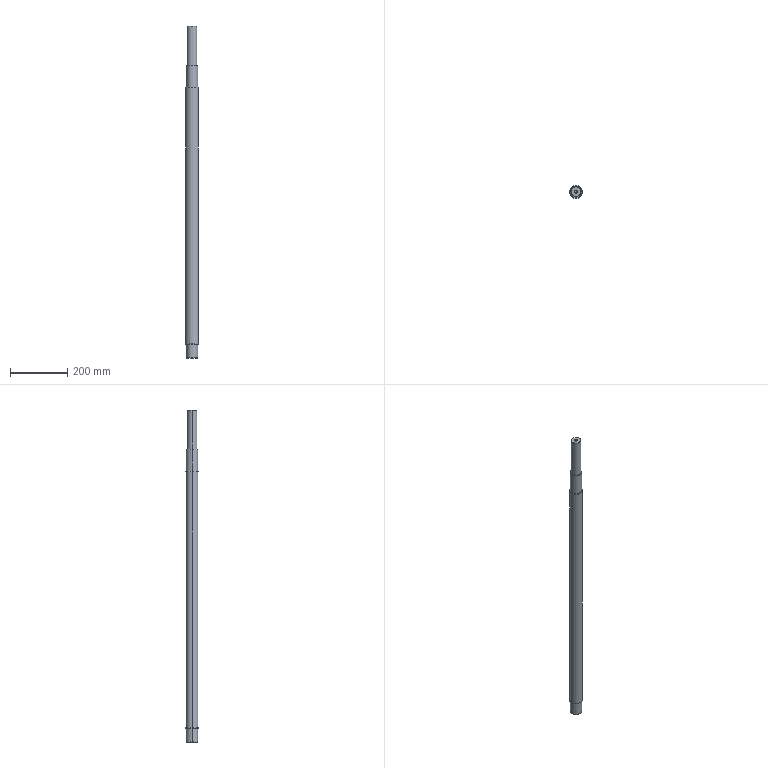Part | SolidWorks | features ICE 4, Chamfer 2, HoleWzd 2, Extrusion 1, Fillet 1 | 1 solid | 39 faces | box 45 x 45 x 1164 mm | volume 1714375 mm3 | cylinder 15 | cone 14 | plane 8 | torus 2 | commonest cylinder face diameters 40 x4 10 x3 8.5 x2 10.2 x2 35 x2 45 x2
STEP:
#1=CARTESIAN_POINT('',(-21.,0.,0.));
#2=VERTEX_POINT('',#1);
#3=CARTESIAN_POINT('',(21.,0.,0.));
#4=VERTEX_POINT('',#3);
#5=CARTESIAN_POINT('',(0.,0.,0.));
#6=DIRECTION('',(0.,0.,1.));
#7=DIRECTION('',(1.,0.,0.));
#8=AXIS2_PLACEMENT_3D('',#5,#6,#7);
#9=CIRCLE('',#8,21.);
#10=EDGE_CURVE('',#2,#4,#9,.T.);
#11=ORIENTED_EDGE('',*,*,#10,.F.);
#12=CARTESIAN_POINT('',(-20.,0.,-1.));
#13=VERTEX_POINT('',#12);
#14=CARTESIAN_POINT('',(-21.,0.,-1.));
#15=DIRECTION('',(0.,1.,0.));
#16=DIRECTION('',(-1.,0.,0.));
#17=AXIS2_PLACEMENT_3D('',#14,#15,#16);
#18=CIRCLE('',#17,1.);
#19=EDGE_CURVE('',#2,#13,#18,.T.);
#20=ORIENTED_EDGE('',*,*,#19,.T.);
#21=CARTESIAN_POINT('',(20.,0.,-1.));
#22=VERTEX_POINT('',#21);
#23=CARTESIAN_POINT('',(0.,0.,-1.));
#24=DIRECTION('',(0.,0.,-1.));
#25=DIRECTION('',(1.,0.,0.));
#26=AXIS2_PLACEMENT_3D('',#23,#24,#25);
#27=CIRCLE('',#26,20.);
#28=EDGE_CURVE('',#22,#13,#27,.T.);
#29=ORIENTED_EDGE('',*,*,#28,.F.);
#30=CARTESIAN_POINT('',(21.,0.,-1.));
#31=DIRECTION('',(0.,-1.,0.));
#32=DIRECTION('',(0.,0.,-1.));
#33=AXIS2_PLACEMENT_3D('',#30,#31,#32);
#34=CIRCLE('',#33,1.);
#35=EDGE_CURVE('',#4,#22,#34,.T.);
#36=ORIENTED_EDGE('',*,*,#35,.F.);
#37=EDGE_LOOP('',(#11,#20,#29,#36));
#38=FACE_OUTER_BOUND('',#37,.T.);
#39=CARTESIAN_POINT('',(0.,0.,-1.));
#40=DIRECTION('',(0.,0.,1.));
#41=DIRECTION('',(1.,0.,0.));
#42=AXIS2_PLACEMENT_3D('',#39,#40,#41);
#43=TOROIDAL_SURFACE('',#42,21.,1.);
#44=ADVANCED_FACE('',(#38),#43,.F.);
#45=CARTESIAN_POINT('',(-22.098,0.,0.));
#46=VERTEX_POINT('',#45);
#47=CARTESIAN_POINT('',(22.098,0.,0.));
#48=VERTEX_POINT('',#47);
#49=CARTESIAN_POINT('',(0.,0.,0.));
#50=DIRECTION('',(0.,0.,-1.));
#51=DIRECTION('',(1.,0.,0.));
#52=AXIS2_PLACEMENT_3D('',#49,#50,#51);
#53=CIRCLE('',#52,22.098);
#54=EDGE_CURVE('',#46,#48,#53,.T.);
#55=ORIENTED_EDGE('',*,*,#54,.F.);
#56=CARTESIAN_POINT('',(-22.5,0.,1.5));
#57=VERTEX_POINT('',#56);
#58=CARTESIAN_POINT('',(-22.5,0.,1.5));
#59=DIRECTION('',(-0.2588,0.,0.9659));
#60=VECTOR('',#59,1000.);
#61=LINE('',#58,#60);
#62=EDGE_CURVE('',#46,#57,#61,.T.);
#63=ORIENTED_EDGE('',*,*,#62,.T.);
#64=CARTESIAN_POINT('',(22.5,0.,1.5));
#65=VERTEX_POINT('',#64);
#66=CARTESIAN_POINT('',(0.,0.,1.5));
#67=DIRECTION('',(0.,0.,1.));
#68=DIRECTION('',(1.,0.,0.));
#69=AXIS2_PLACEMENT_3D('',#66,#67,#68);
#70=CIRCLE('',#69,22.5);
#71=EDGE_CURVE('',#65,#57,#70,.T.);
#72=ORIENTED_EDGE('',*,*,#71,.F.);
#73=CARTESIAN_POINT('',(22.5,0.,1.5));
#74=DIRECTION('',(0.2588,0.,0.9659));
#75=VECTOR('',#74,1000.);
#76=LINE('',#73,#75);
#77=EDGE_CURVE('',#48,#65,#76,.T.);
#78=ORIENTED_EDGE('',*,*,#77,.F.);
#79=EDGE_LOOP('',(#55,#63,#72,#78));
#80=FACE_OUTER_BOUND('',#79,.T.);
#81=CARTESIAN_POINT('',(0.,0.,1.5));
#82=DIRECTION('',(0.,0.,1.));
#83=DIRECTION('',(1.,0.,0.));
#84=AXIS2_PLACEMENT_3D('',#81,#82,#83);
#85=CONICAL_SURFACE('',#84,22.5,0.2618);
#86=ADVANCED_FACE('',(#80),#85,.T.);
#87=CARTESIAN_POINT('',(4.25,0.,-24.));
#88=VERTEX_POINT('',#87);
#89=CARTESIAN_POINT('',(-4.25,0.,-24.));
#90=VERTEX_POINT('',#89);
#91=CARTESIAN_POINT('',(0.,0.,-24.));
#92=DIRECTION('',(0.,0.,-1.));
#93=DIRECTION('',(-1.,0.,0.));
#94=AXIS2_PLACEMENT_3D('',#91,#92,#93);
#95=CIRCLE('',#94,4.25);
#96=EDGE_CURVE('',#88,#90,#95,.T.);
#97=ORIENTED_EDGE('',*,*,#96,.F.);
#98=CARTESIAN_POINT('',(4.25,0.,-48.5));
#99=VERTEX_POINT('',#98);
#100=CARTESIAN_POINT('',(4.25,0.,-48.5));
#101=DIRECTION('',(0.,0.,-1.));
#102=VECTOR('',#101,1000.);
#103=LINE('',#100,#102);
#104=EDGE_CURVE('',#88,#99,#103,.T.);
#105=ORIENTED_EDGE('',*,*,#104,.T.);
#106=CARTESIAN_POINT('',(-4.25,0.,-48.5));
#107=VERTEX_POINT('',#106);
#108=CARTESIAN_POINT('',(0.,0.,-48.5));
#109=DIRECTION('',(0.,0.,-1.));
#110=DIRECTION('',(-1.,0.,0.));
#111=AXIS2_PLACEMENT_3D('',#108,#109,#110);
#112=CIRCLE('',#111,4.25);
#113=EDGE_CURVE('',#99,#107,#112,.T.);
#114=ORIENTED_EDGE('',*,*,#113,.T.);
#115=CARTESIAN_POINT('',(-4.25,0.,-48.5));
#116=DIRECTION('',(0.,0.,-1.));
#117=VECTOR('',#116,1000.);
#118=LINE('',#115,#117);
#119=EDGE_CURVE('',#90,#107,#118,.T.);
#120=ORIENTED_EDGE('',*,*,#119,.F.);
#121=EDGE_LOOP('',(#97,#105,#114,#120));
#122=FACE_OUTER_BOUND('',#121,.T.);
#123=CARTESIAN_POINT('',(0.,0.,-48.5));
#124=DIRECTION('',(0.,0.,-1.));
#125=DIRECTION('',(-1.,0.,0.));
#126=AXIS2_PLACEMENT_3D('',#123,#124,#125);
#127=CYLINDRICAL_SURFACE('',#126,4.25);
#128=ADVANCED_FACE('',(#122),#127,.F.);
#129=CARTESIAN_POINT('',(0.,0.,-21.446));
#130=VERTEX_POINT('',#129);
#131=CARTESIAN_POINT('',(-4.25,0.,-24.));
#132=DIRECTION('',(-0.8572,0.,-0.515));
#133=VECTOR('',#132,1000.);
#134=LINE('',#131,#133);
#135=EDGE_CURVE('',#130,#90,#134,.T.);
#136=ORIENTED_EDGE('',*,*,#135,.F.);
#137=CARTESIAN_POINT('',(4.25,0.,-24.));
#138=DIRECTION('',(0.8572,0.,-0.515));
#139=VECTOR('',#138,1000.);
#140=LINE('',#137,#139);
#141=EDGE_CURVE('',#130,#88,#140,.T.);
#142=ORIENTED_EDGE('',*,*,#141,.T.);
#143=ORIENTED_EDGE('',*,*,#96,.T.);
#144=EDGE_LOOP('',(#136,#142,#143));
#145=FACE_OUTER_BOUND('',#144,.T.);
#146=CARTESIAN_POINT('',(0.,0.,-24.));
#147=DIRECTION('',(0.,0.,-1.));
#148=DIRECTION('',(-1.,0.,0.));
#149=AXIS2_PLACEMENT_3D('',#146,#147,#148);
#150=CONICAL_SURFACE('',#149,4.25,1.03);
#151=ADVANCED_FACE('',(#145),#150,.F.);
#152=CARTESIAN_POINT('',(-5.1,0.,1085.75));
#153=VERTEX_POINT('',#152);
#154=CARTESIAN_POINT('',(5.1,0.,1085.75));
#155=VERTEX_POINT('',#154);
#156=CARTESIAN_POINT('',(0.,0.,1085.75));
#157=DIRECTION('',(0.,0.,1.));
#158=DIRECTION('',(1.,0.,0.));
#159=AXIS2_PLACEMENT_3D('',#156,#157,#158);
#160=CIRCLE('',#159,5.1);
#161=EDGE_CURVE('',#153,#155,#160,.T.);
#162=ORIENTED_EDGE('',*,*,#161,.F.);
#163=CARTESIAN_POINT('',(-5.1,0.,1115.));
#164=VERTEX_POINT('',#163);
#165=CARTESIAN_POINT('',(-5.1,0.,1115.));
#166=DIRECTION('',(0.,0.,1.));
#167=VECTOR('',#166,1000.);
#168=LINE('',#165,#167);
#169=EDGE_CURVE('',#153,#164,#168,.T.);
#170=ORIENTED_EDGE('',*,*,#169,.T.);
#171=CARTESIAN_POINT('',(5.1,0.,1115.));
#172=VERTEX_POINT('',#171);
#173=CARTESIAN_POINT('',(0.,0.,1115.));
#174=DIRECTION('',(0.,0.,1.));
#175=DIRECTION('',(1.,0.,0.));
#176=AXIS2_PLACEMENT_3D('',#173,#174,#175);
#177=CIRCLE('',#176,5.1);
#178=EDGE_CURVE('',#164,#172,#177,.T.);
#179=ORIENTED_EDGE('',*,*,#178,.T.);
#180=CARTESIAN_POINT('',(5.1,0.,1115.));
#181=DIRECTION('',(0.,0.,1.));
#182=VECTOR('',#181,1000.);
#183=LINE('',#180,#182);
#184=EDGE_CURVE('',#155,#172,#183,.T.);
#185=ORIENTED_EDGE('',*,*,#184,.F.);
#186=EDGE_LOOP('',(#162,#170,#179,#185));
#187=FACE_OUTER_BOUND('',#186,.T.);
#188=CARTESIAN_POINT('',(0.,0.,1115.));
#189=DIRECTION('',(0.,0.,1.));
#190=DIRECTION('',(1.,0.,0.));
#191=AXIS2_PLACEMENT_3D('',#188,#189,#190);
#192=CYLINDRICAL_SURFACE('',#191,5.1);
#193=ADVANCED_FACE('',(#187),#192,.F.);
#194=CARTESIAN_POINT('',(0.,0.,1082.686));
#195=VERTEX_POINT('',#194);
#196=CARTESIAN_POINT('',(5.1,0.,1085.75));
#197=DIRECTION('',(0.8572,0.,0.515));
#198=VECTOR('',#197,1000.);
#199=LINE('',#196,#198);
#200=EDGE_CURVE('',#195,#155,#199,.T.);
#201=ORIENTED_EDGE('',*,*,#200,.F.);
#202=CARTESIAN_POINT('',(-5.1,0.,1085.75));
#203=DIRECTION('',(-0.8572,0.,0.515));
#204=VECTOR('',#203,1000.);
#205=LINE('',#202,#204);
#206=EDGE_CURVE('',#195,#153,#205,.T.);
#207=ORIENTED_EDGE('',*,*,#206,.T.);
#208=ORIENTED_EDGE('',*,*,#161,.T.);
#209=EDGE_LOOP('',(#201,#207,#208));
#210=FACE_OUTER_BOUND('',#209,.T.);
#211=CARTESIAN_POINT('',(0.,0.,1085.75));
#212=DIRECTION('',(0.,0.,1.));
#213=DIRECTION('',(1.,0.,0.));
#214=AXIS2_PLACEMENT_3D('',#211,#212,#213);
#215=CONICAL_SURFACE('',#214,5.1,1.03);
#216=ADVANCED_FACE('',(#210),#215,.F.);
#217=CARTESIAN_POINT('',(0.,12.5,1078.));
#218=VERTEX_POINT('',#217);
#219=CARTESIAN_POINT('',(5.,12.5,1073.));
#220=VERTEX_POINT('',#219);
#221=CARTESIAN_POINT('',(0.,12.5,1073.));
#222=DIRECTION('',(0.,1.,0.));
#223=DIRECTION('',(0.,0.,1.));
#224=AXIS2_PLACEMENT_3D('',#221,#222,#223);
#225=CIRCLE('',#224,5.);
#226=EDGE_CURVE('',#218,#220,#225,.T.);
#227=ORIENTED_EDGE('',*,*,#226,.F.);
#228=CARTESIAN_POINT('',(0.,17.5,1078.));
#229=VERTEX_POINT('',#228);
#230=CARTESIAN_POINT('',(0.,12.5,1078.));
#231=DIRECTION('',(0.,1.,0.));
#232=VECTOR('',#231,1000.);
#233=LINE('',#230,#232);
#234=EDGE_CURVE('',#218,#229,#233,.T.);
#235=ORIENTED_EDGE('',*,*,#234,.T.);
#236=CARTESIAN_POINT('',(5.,16.771,1073.));
#237=VERTEX_POINT('',#236);
#238=CARTESIAN_POINT('',(5.,16.771,1073.));
#239=CARTESIAN_POINT('',(5.,16.771,1073.332));
#240=CARTESIAN_POINT('',(4.967,16.78,1073.659));
#241=CARTESIAN_POINT('',(4.839,16.818,1074.3));
#242=CARTESIAN_POINT('',(4.742,16.846,1074.619));
#243=CARTESIAN_POINT('',(4.49,16.915,1075.224));
#244=CARTESIAN_POINT('',(4.337,16.955,1075.51));
#245=CARTESIAN_POINT('',(3.974,17.044,1076.052));
#246=CARTESIAN_POINT('',(3.764,17.092,1076.308));
#247=CARTESIAN_POINT('',(3.305,17.187,1076.766));
#248=CARTESIAN_POINT('',(3.054,17.234,1076.973));
#249=CARTESIAN_POINT('',(2.507,17.322,1077.338));
#250=CARTESIAN_POINT('',(2.219,17.361,1077.492));
#251=CARTESIAN_POINT('',(1.768,17.411,1077.68));
#252=CARTESIAN_POINT('',(1.614,17.426,1077.735));
#253=CARTESIAN_POINT('',(1.3,17.452,1077.831));
#254=CARTESIAN_POINT('',(1.139,17.464,1077.871));
#255=CARTESIAN_POINT('',(0.6539,17.491,1077.968));
#256=CARTESIAN_POINT('',(0.3282,17.5,1078.));
#257=CARTESIAN_POINT('',(0.,17.5,1078.));
#258=B_SPLINE_CURVE_WITH_KNOTS('',3,(#238,#239,#240,#241,#242,#243,#244,#245,#246,#247,#248,#249,#250,#251,#252,#253,#254,#255,#256,#257),.UNSPECIFIED.,.F.,.F.,(4,2,2,2,2,2,2,2,2,4),(0.,0.0009824,0.001965,0.002947,0.00393,0.004912,0.005894,0.006386,0.006877,0.007859),.UNSPECIFIED.);
#259=EDGE_CURVE('',#237,#229,#258,.T.);
#260=ORIENTED_EDGE('',*,*,#259,.F.);
#261=CARTESIAN_POINT('',(5.,12.5,1073.));
#262=DIRECTION('',(0.,1.,0.));
#263=VECTOR('',#262,1000.);
#264=LINE('',#261,#263);
#265=EDGE_CURVE('',#220,#237,#264,.T.);
#266=ORIENTED_EDGE('',*,*,#265,.F.);
#267=EDGE_LOOP('',(#227,#235,#260,#266));
#268=FACE_OUTER_BOUND('',#267,.T.);
#269=CARTESIAN_POINT('',(0.,12.5,1073.));
#270=DIRECTION('',(0.,1.,0.));
#271=DIRECTION('',(0.,0.,1.));
#272=AXIS2_PLACEMENT_3D('',#269,#270,#271);
#273=CYLINDRICAL_SURFACE('',#272,5.);
#274=ADVANCED_FACE('',(#268),#273,.F.);
#275=CARTESIAN_POINT('',(22.098,0.,900.));
#276=VERTEX_POINT('',#275);
#277=CARTESIAN_POINT('',(-22.098,0.,900.));
#278=VERTEX_POINT('',#277);
#279=CARTESIAN_POINT('',(0.,0.,900.));
#280=DIRECTION('',(0.,0.,1.));
#281=DIRECTION('',(1.,0.,0.));
#282=AXIS2_PLACEMENT_3D('',#279,#280,#281);
#283=CIRCLE('',#282,22.098);
#284=EDGE_CURVE('',#276,#278,#283,.T.);
#285=ORIENTED_EDGE('',*,*,#284,.F.);
#286=CARTESIAN_POINT('',(22.5,0.,898.5));
#287=VERTEX_POINT('',#286);
#288=CARTESIAN_POINT('',(22.098,0.,900.));
#289=DIRECTION('',(0.2588,0.,-0.9659));
#290=VECTOR('',#289,1000.);
#291=LINE('',#288,#290);
#292=EDGE_CURVE('',#276,#287,#291,.T.);
#293=ORIENTED_EDGE('',*,*,#292,.T.);
#294=CARTESIAN_POINT('',(-22.5,0.,898.5));
#295=VERTEX_POINT('',#294);
#296=CARTESIAN_POINT('',(0.,0.,898.5));
#297=DIRECTION('',(0.,0.,-1.));
#298=DIRECTION('',(1.,0.,0.));
#299=AXIS2_PLACEMENT_3D('',#296,#297,#298);
#300=CIRCLE('',#299,22.5);
#301=EDGE_CURVE('',#295,#287,#300,.T.);
#302=ORIENTED_EDGE('',*,*,#301,.F.);
#303=CARTESIAN_POINT('',(-22.098,0.,900.));
#304=DIRECTION('',(-0.2588,0.,-0.9659));
#305=VECTOR('',#304,1000.);
#306=LINE('',#303,#305);
#307=EDGE_CURVE('',#278,#295,#306,.T.);
#308=ORIENTED_EDGE('',*,*,#307,.F.);
#309=EDGE_LOOP('',(#285,#293,#302,#308));
#310=FACE_OUTER_BOUND('',#309,.T.);
#311=CARTESIAN_POINT('',(0.,0.,900.));
#312=DIRECTION('',(0.,0.,-1.));
#313=DIRECTION('',(-1.,0.,0.));
#314=AXIS2_PLACEMENT_3D('',#311,#312,#313);
#315=CONICAL_SURFACE('',#314,22.098,0.2618);
#316=ADVANCED_FACE('',(#310),#315,.T.);
#317=CARTESIAN_POINT('',(19.598,0.,978.));
#318=VERTEX_POINT('',#317);
#319=CARTESIAN_POINT('',(-19.598,0.,978.));
#320=VERTEX_POINT('',#319);
#321=CARTESIAN_POINT('',(0.,0.,978.));
#322=DIRECTION('',(0.,0.,1.));
#323=DIRECTION('',(1.,0.,0.));
#324=AXIS2_PLACEMENT_3D('',#321,#322,#323);
#325=CIRCLE('',#324,19.598);
#326=EDGE_CURVE('',#318,#320,#325,.T.);
#327=ORIENTED_EDGE('',*,*,#326,.F.);
#328=CARTESIAN_POINT('',(20.,0.,976.5));
#329=VERTEX_POINT('',#328);
#330=CARTESIAN_POINT('',(19.598,0.,978.));
#331=DIRECTION('',(0.2588,0.,-0.9659));
#332=VECTOR('',#331,1000.);
#333=LINE('',#330,#332);
#334=EDGE_CURVE('',#318,#329,#333,.T.);
#335=ORIENTED_EDGE('',*,*,#334,.T.);
#336=CARTESIAN_POINT('',(-20.,0.,976.5));
#337=VERTEX_POINT('',#336);
#338=CARTESIAN_POINT('',(0.,0.,976.5));
#339=DIRECTION('',(0.,0.,-1.));
#340=DIRECTION('',(1.,0.,0.));
#341=AXIS2_PLACEMENT_3D('',#338,#339,#340);
#342=CIRCLE('',#341,20.);
#343=EDGE_CURVE('',#337,#329,#342,.T.);
#344=ORIENTED_EDGE('',*,*,#343,.F.);
#345=CARTESIAN_POINT('',(-19.598,0.,978.));
#346=DIRECTION('',(-0.2588,0.,-0.9659));
#347=VECTOR('',#346,1000.);
#348=LINE('',#345,#347);
#349=EDGE_CURVE('',#320,#337,#348,.T.);
#350=ORIENTED_EDGE('',*,*,#349,.F.);
#351=EDGE_LOOP('',(#327,#335,#344,#350));
#352=FACE_OUTER_BOUND('',#351,.T.);
#353=CARTESIAN_POINT('',(0.,0.,978.));
#354=DIRECTION('',(0.,0.,-1.));
#355=DIRECTION('',(-1.,0.,0.));
#356=AXIS2_PLACEMENT_3D('',#353,#354,#355);
#357=CONICAL_SURFACE('',#356,19.598,0.2618);
#358=ADVANCED_FACE('',(#352),#357,.T.);
#359=CARTESIAN_POINT('',(17.098,0.,1115.));
#360=VERTEX_POINT('',#359);
#361=CARTESIAN_POINT('',(-17.098,0.,1115.));
#362=VERTEX_POINT('',#361);
#363=CARTESIAN_POINT('',(0.,0.,1115.));
#364=DIRECTION('',(0.,0.,1.));
#365=DIRECTION('',(1.,0.,0.));
#366=AXIS2_PLACEMENT_3D('',#363,#364,#365);
#367=CIRCLE('',#366,17.098);
#368=EDGE_CURVE('',#360,#362,#367,.T.);
#369=ORIENTED_EDGE('',*,*,#368,.F.);
#370=CARTESIAN_POINT('',(17.5,0.,1113.5));
#371=VERTEX_POINT('',#370);
#372=CARTESIAN_POINT('',(17.098,0.,1115.));
#373=DIRECTION('',(0.2588,0.,-0.9659));
#374=VECTOR('',#373,1000.);
#375=LINE('',#372,#374);
#376=EDGE_CURVE('',#360,#371,#375,.T.);
#377=ORIENTED_EDGE('',*,*,#376,.T.);
#378=CARTESIAN_POINT('',(-17.5,0.,1113.5));
#379=VERTEX_POINT('',#378);
#380=CARTESIAN_POINT('',(0.,0.,1113.5));
#381=DIRECTION('',(0.,0.,-1.));
#382=DIRECTION('',(1.,0.,0.));
#383=AXIS2_PLACEMENT_3D('',#380,#381,#382);
#384=CIRCLE('',#383,17.5);
#385=EDGE_CURVE('',#379,#371,#384,.T.);
#386=ORIENTED_EDGE('',*,*,#385,.F.);
#387=CARTESIAN_POINT('',(-17.098,0.,1115.));
#388=DIRECTION('',(-0.2588,0.,-0.9659));
#389=VECTOR('',#388,1000.);
#390=LINE('',#387,#389);
#391=EDGE_CURVE('',#362,#379,#390,.T.);
#392=ORIENTED_EDGE('',*,*,#391,.F.);
#393=EDGE_LOOP('',(#369,#377,#386,#392));
#394=FACE_OUTER_BOUND('',#393,.T.);
#395=CARTESIAN_POINT('',(0.,0.,1115.));
#396=DIRECTION('',(0.,0.,-1.));
#397=DIRECTION('',(-1.,0.,0.));
#398=AXIS2_PLACEMENT_3D('',#395,#396,#397);
#399=CONICAL_SURFACE('',#398,17.098,0.2618);
#400=ADVANCED_FACE('',(#394),#399,.T.);
#401=CARTESIAN_POINT('',(-19.598,0.,-48.5));
#402=VERTEX_POINT('',#401);
#403=CARTESIAN_POINT('',(19.598,0.,-48.5));
#404=VERTEX_POINT('',#403);
#405=CARTESIAN_POINT('',(0.,0.,-48.5));
#406=DIRECTION('',(0.,0.,-1.));
#407=DIRECTION('',(-1.,0.,0.));
#408=AXIS2_PLACEMENT_3D('',#405,#406,#407);
#409=CIRCLE('',#408,19.598);
#410=EDGE_CURVE('',#402,#404,#409,.T.);
#411=ORIENTED_EDGE('',*,*,#410,.F.);
#412=CARTESIAN_POINT('',(-20.,0.,-47.));
#413=VERTEX_POINT('',#412);
#414=CARTESIAN_POINT('',(-19.598,0.,-48.5));
#415=DIRECTION('',(-0.2588,0.,0.9659));
#416=VECTOR('',#415,1000.);
#417=LINE('',#414,#416);
#418=EDGE_CURVE('',#402,#413,#417,.T.);
#419=ORIENTED_EDGE('',*,*,#418,.T.);
#420=CARTESIAN_POINT('',(20.,0.,-47.));
#421=VERTEX_POINT('',#420);
#422=CARTESIAN_POINT('',(0.,0.,-47.));
#423=DIRECTION('',(0.,0.,1.));
#424=DIRECTION('',(-1.,0.,0.));
#425=AXIS2_PLACEMENT_3D('',#422,#423,#424);
#426=CIRCLE('',#425,20.);
#427=EDGE_CURVE('',#421,#413,#426,.T.);
#428=ORIENTED_EDGE('',*,*,#427,.F.);
#429=CARTESIAN_POINT('',(19.598,0.,-48.5));
#430=DIRECTION('',(0.2588,0.,0.9659));
#431=VECTOR('',#430,1000.);
#432=LINE('',#429,#431);
#433=EDGE_CURVE('',#404,#421,#432,.T.);
#434=ORIENTED_EDGE('',*,*,#433,.F.);
#435=EDGE_LOOP('',(#411,#419,#428,#434));
#436=FACE_OUTER_BOUND('',#435,.T.);
#437=CARTESIAN_POINT('',(0.,0.,-48.5));
#438=DIRECTION('',(0.,0.,1.));
#439=DIRECTION('',(1.,0.,0.));
#440=AXIS2_PLACEMENT_3D('',#437,#438,#439);
#441=CONICAL_SURFACE('',#440,19.598,0.2618);
#442=ADVANCED_FACE('',(#436),#441,.T.);
#443=ORIENTED_EDGE('',*,*,#427,.T.);
#444=CARTESIAN_POINT('',(-20.,0.,-48.5));
#445=DIRECTION('',(0.,0.,1.));
#446=VECTOR('',#445,1000.);
#447=LINE('',#444,#446);
#448=EDGE_CURVE('',#413,#13,#447,.T.);
#449=ORIENTED_EDGE('',*,*,#448,.T.);
#450=CARTESIAN_POINT('',(0.,0.,-1.));
#451=DIRECTION('',(0.,0.,-1.));
#452=DIRECTION('',(1.,0.,0.));
#453=AXIS2_PLACEMENT_3D('',#450,#451,#452);
#454=CIRCLE('',#453,20.);
#455=EDGE_CURVE('',#13,#22,#454,.T.);
#456=ORIENTED_EDGE('',*,*,#455,.T.);
#457=CARTESIAN_POINT('',(20.,0.,-48.5));
#458=DIRECTION('',(0.,0.,1.));
#459=VECTOR('',#458,1000.);
#460=LINE('',#457,#459);
#461=EDGE_CURVE('',#421,#22,#460,.T.);
#462=ORIENTED_EDGE('',*,*,#461,.F.);
#463=EDGE_LOOP('',(#443,#449,#456,#462));
#464=FACE_OUTER_BOUND('',#463,.T.);
#465=CARTESIAN_POINT('',(0.,0.,-48.5));
#466=DIRECTION('',(0.,0.,1.));
#467=DIRECTION('',(1.,0.,0.));
#468=AXIS2_PLACEMENT_3D('',#465,#466,#467);
#469=CYLINDRICAL_SURFACE('',#468,20.);
#470=ADVANCED_FACE('',(#464),#469,.T.);
#471=CARTESIAN_POINT('',(5.,16.771,1003.));
#472=VERTEX_POINT('',#471);
#473=CARTESIAN_POINT('',(5.,16.771,1115.));
#474=DIRECTION('',(0.,0.,-1.));
#475=VECTOR('',#474,1000.);
#476=LINE('',#473,#475);
#477=EDGE_CURVE('',#237,#472,#476,.T.);
#478=ORIENTED_EDGE('',*,*,#477,.F.);
#479=ORIENTED_EDGE('',*,*,#259,.T.);
#480=CARTESIAN_POINT('',(-5.,16.771,1073.));
#481=VERTEX_POINT('',#480);
#482=CARTESIAN_POINT('',(0.,17.5,1078.));
#483=CARTESIAN_POINT('',(-0.3278,17.5,1078.));
#484=CARTESIAN_POINT('',(-0.6608,17.49,1077.967));
#485=CARTESIAN_POINT('',(-1.303,17.454,1077.838));
#486=CARTESIAN_POINT('',(-1.615,17.428,1077.743));
#487=CARTESIAN_POINT('',(-2.222,17.361,1077.491));
#488=CARTESIAN_POINT('',(-2.512,17.321,1077.335));
#489=CARTESIAN_POINT('',(-3.051,17.234,1076.974));
#490=CARTESIAN_POINT('',(-3.305,17.187,1076.766));
#491=CARTESIAN_POINT('',(-3.767,17.091,1076.304));
#492=CARTESIAN_POINT('',(-3.972,17.044,1076.054));
#493=CARTESIAN_POINT('',(-4.334,16.956,1075.514));
#494=CARTESIAN_POINT('',(-4.491,16.914,1075.222));
#495=CARTESIAN_POINT('',(-4.742,16.846,1074.62));
#496=CARTESIAN_POINT('',(-4.837,16.818,1074.308));
#497=CARTESIAN_POINT('',(-4.967,16.781,1073.664));
#498=CARTESIAN_POINT('',(-5.,16.771,1073.332));
#499=CARTESIAN_POINT('',(-5.,16.771,1073.));
#500=B_SPLINE_CURVE_WITH_KNOTS('',3,(#482,#483,#484,#485,#486,#487,#488,#489,#490,#491,#492,#493,#494,#495,#496,#497,#498,#499),.UNSPECIFIED.,.F.,.F.,(4,2,2,2,2,2,2,2,4),(0.007859,0.008841,0.009822,0.0108,0.01178,0.01277,0.01375,0.01473,0.01571),.UNSPECIFIED.);
#501=EDGE_CURVE('',#229,#481,#500,.T.);
#502=ORIENTED_EDGE('',*,*,#501,.T.);
#503=CARTESIAN_POINT('',(-5.,16.771,1003.));
#504=VERTEX_POINT('',#503);
#505=CARTESIAN_POINT('',(-5.,16.771,1115.));
#506=DIRECTION('',(0.,0.,-1.));
#507=VECTOR('',#506,1000.);
#508=LINE('',#505,#507);
#509=EDGE_CURVE('',#481,#504,#508,.T.);
#510=ORIENTED_EDGE('',*,*,#509,.T.);
#511=CARTESIAN_POINT('',(-5.,16.771,1003.));
#512=CARTESIAN_POINT('',(-5.,16.771,1002.668));
#513=CARTESIAN_POINT('',(-4.967,16.78,1002.342));
#514=CARTESIAN_POINT('',(-4.839,16.818,1001.7));
#515=CARTESIAN_POINT('',(-4.742,16.846,1001.382));
#516=CARTESIAN_POINT('',(-4.491,16.914,1000.778));
#517=CARTESIAN_POINT('',(-4.337,16.955,1000.491));
#518=CARTESIAN_POINT('',(-3.975,17.044,999.949));
#519=CARTESIAN_POINT('',(-3.765,17.092,999.694));
#520=CARTESIAN_POINT('',(-3.306,17.186,999.235));
#521=CARTESIAN_POINT('',(-3.056,17.233,999.029));
#522=CARTESIAN_POINT('',(-2.51,17.321,998.663));
#523=CARTESIAN_POINT('',(-2.222,17.361,998.509));
#524=CARTESIAN_POINT('',(-1.771,17.411,998.321));
#525=CARTESIAN_POINT('',(-1.618,17.426,998.266));
#526=CARTESIAN_POINT('',(-1.304,17.452,998.17));
#527=CARTESIAN_POINT('',(-1.143,17.463,998.13));
#528=CARTESIAN_POINT('',(-0.6583,17.491,998.033));
#529=CARTESIAN_POINT('',(-0.3328,17.5,998.));
#530=CARTESIAN_POINT('',(0.3232,17.5,998.));
#531=CARTESIAN_POINT('',(0.6564,17.491,998.032));
#532=CARTESIAN_POINT('',(1.299,17.455,998.161));
#533=CARTESIAN_POINT('',(1.612,17.428,998.255));
#534=CARTESIAN_POINT('',(2.219,17.361,998.507));
#535=CARTESIAN_POINT('',(2.509,17.321,998.663));
#536=CARTESIAN_POINT('',(3.049,17.235,999.024));
#537=CARTESIAN_POINT('',(3.303,17.187,999.232));
#538=CARTESIAN_POINT('',(3.765,17.092,999.694));
#539=CARTESIAN_POINT('',(3.971,17.045,999.945));
#540=CARTESIAN_POINT('',(4.333,16.956,1000.484));
#541=CARTESIAN_POINT('',(4.49,16.915,1000.777));
#542=CARTESIAN_POINT('',(4.741,16.846,1001.379));
#543=CARTESIAN_POINT('',(4.837,16.818,1001.691));
#544=CARTESIAN_POINT('',(4.967,16.781,1002.336));
#545=CARTESIAN_POINT('',(5.,16.771,1002.668));
#546=CARTESIAN_POINT('',(5.,16.771,1003.));
#547=B_SPLINE_CURVE_WITH_KNOTS('',3,(#511,#512,#513,#514,#515,#516,#517,#518,#519,#520,#521,#522,#523,#524,#525,#526,#527,#528,#529,#530,#531,#532,#533,#534,#535,#536,#537,#538,#539,#540,#541,#542,#543,#544,#545,#546),.UNSPECIFIED.,.F.,.F.,(4,2,2,2,2,2,2,2,2,2,2,2,2,2,2,2,2,4),(0.,0.0009818,0.001964,0.002945,0.003927,0.004909,0.005891,0.006382,0.006873,0.007855,0.008836,0.009818,0.0108,0.01178,0.01276,0.01375,0.01473,0.01571),.UNSPECIFIED.);
#548=EDGE_CURVE('',#504,#472,#547,.T.);
#549=ORIENTED_EDGE('',*,*,#548,.T.);
#550=EDGE_LOOP('',(#478,#479,#502,#510,#549));
#551=FACE_BOUND('',#550,.T.);
#552=ORIENTED_EDGE('',*,*,#385,.T.);
#553=CARTESIAN_POINT('',(17.5,0.,978.));
#554=VERTEX_POINT('',#553);
#555=CARTESIAN_POINT('',(17.5,0.,1115.));
#556=DIRECTION('',(0.,0.,-1.));
#557=VECTOR('',#556,1000.);
#558=LINE('',#555,#557);
#559=EDGE_CURVE('',#371,#554,#558,.T.);
#560=ORIENTED_EDGE('',*,*,#559,.T.);
#561=CARTESIAN_POINT('',(-17.5,0.,978.));
#562=VERTEX_POINT('',#561);
#563=CARTESIAN_POINT('',(0.,0.,978.));
#564=DIRECTION('',(0.,0.,1.));
#565=DIRECTION('',(1.,0.,0.));
#566=AXIS2_PLACEMENT_3D('',#563,#564,#565);
#567=CIRCLE('',#566,17.5);
#568=EDGE_CURVE('',#554,#562,#567,.T.);
#569=ORIENTED_EDGE('',*,*,#568,.T.);
#570=CARTESIAN_POINT('',(-17.5,0.,1115.));
#571=DIRECTION('',(0.,0.,-1.));
#572=VECTOR('',#571,1000.);
#573=LINE('',#570,#572);
#574=EDGE_CURVE('',#379,#562,#573,.T.);
#575=ORIENTED_EDGE('',*,*,#574,.F.);
#576=EDGE_LOOP('',(#552,#560,#569,#575));
#577=FACE_OUTER_BOUND('',#576,.T.);
#578=CARTESIAN_POINT('',(0.,0.,1115.));
#579=DIRECTION('',(0.,0.,-1.));
#580=DIRECTION('',(-1.,0.,0.));
#581=AXIS2_PLACEMENT_3D('',#578,#579,#580);
#582=CYLINDRICAL_SURFACE('',#581,17.5);
#583=ADVANCED_FACE('',(#551,#577),#582,.T.);
#584=ORIENTED_EDGE('',*,*,#343,.T.);
#585=CARTESIAN_POINT('',(20.,0.,900.));
#586=VERTEX_POINT('',#585);
#587=CARTESIAN_POINT('',(20.,0.,978.));
#588=DIRECTION('',(0.,0.,-1.));
#589=VECTOR('',#588,1000.);
#590=LINE('',#587,#589);
#591=EDGE_CURVE('',#329,#586,#590,.T.);
#592=ORIENTED_EDGE('',*,*,#591,.T.);
#593=CARTESIAN_POINT('',(-20.,0.,900.));
#594=VERTEX_POINT('',#593);
#595=CARTESIAN_POINT('',(0.,0.,900.));
#596=DIRECTION('',(0.,0.,1.));
#597=DIRECTION('',(1.,0.,0.));
#598=AXIS2_PLACEMENT_3D('',#595,#596,#597);
#599=CIRCLE('',#598,20.);
#600=EDGE_CURVE('',#586,#594,#599,.T.);
#601=ORIENTED_EDGE('',*,*,#600,.T.);
#602=CARTESIAN_POINT('',(-20.,0.,978.));
#603=DIRECTION('',(0.,0.,-1.));
#604=VECTOR('',#603,1000.);
#605=LINE('',#602,#604);
#606=EDGE_CURVE('',#337,#594,#605,.T.);
#607=ORIENTED_EDGE('',*,*,#606,.F.);
#608=EDGE_LOOP('',(#584,#592,#601,#607));
#609=FACE_OUTER_BOUND('',#608,.T.);
#610=CARTESIAN_POINT('',(0.,0.,978.));
#611=DIRECTION('',(0.,0.,-1.));
#612=DIRECTION('',(-1.,0.,0.));
#613=AXIS2_PLACEMENT_3D('',#610,#611,#612);
#614=CYLINDRICAL_SURFACE('',#613,20.);
#615=ADVANCED_FACE('',(#609),#614,.T.);
#616=ORIENTED_EDGE('',*,*,#301,.T.);
#617=CARTESIAN_POINT('',(22.5,0.,900.));
#618=DIRECTION('',(0.,0.,-1.));
#619=VECTOR('',#618,1000.);
#620=LINE('',#617,#619);
#621=EDGE_CURVE('',#287,#65,#620,.T.);
#622=ORIENTED_EDGE('',*,*,#621,.T.);
#623=ORIENTED_EDGE('',*,*,#71,.T.);
#624=CARTESIAN_POINT('',(-22.5,0.,900.));
#625=DIRECTION('',(0.,0.,-1.));
#626=VECTOR('',#625,1000.);
#627=LINE('',#624,#626);
#628=EDGE_CURVE('',#295,#57,#627,.T.);
#629=ORIENTED_EDGE('',*,*,#628,.F.);
#630=EDGE_LOOP('',(#616,#622,#623,#629));
#631=FACE_OUTER_BOUND('',#630,.T.);
#632=CARTESIAN_POINT('',(0.,0.,900.));
#633=DIRECTION('',(0.,0.,-1.));
#634=DIRECTION('',(-1.,0.,0.));
#635=AXIS2_PLACEMENT_3D('',#632,#633,#634);
#636=CYLINDRICAL_SURFACE('',#635,22.5);
#637=ADVANCED_FACE('',(#631),#636,.T.);
#638=ORIENTED_EDGE('',*,*,#621,.F.);
#639=CARTESIAN_POINT('',(0.,0.,898.5));
#640=DIRECTION('',(0.,0.,-1.));
#641=DIRECTION('',(1.,0.,0.));
#642=AXIS2_PLACEMENT_3D('',#639,#640,#641);
#643=CIRCLE('',#642,22.5);
#644=EDGE_CURVE('',#287,#295,#643,.T.);
#645=ORIENTED_EDGE('',*,*,#644,.T.);
#646=ORIENTED_EDGE('',*,*,#628,.T.);
#647=CARTESIAN_POINT('',(0.,0.,1.5));
#648=DIRECTION('',(0.,0.,1.));
#649=DIRECTION('',(1.,0.,0.));
#650=AXIS2_PLACEMENT_3D('',#647,#648,#649);
#651=CIRCLE('',#650,22.5);
#652=EDGE_CURVE('',#57,#65,#651,.T.);
#653=ORIENTED_EDGE('',*,*,#652,.T.);
#654=EDGE_LOOP('',(#638,#645,#646,#653));
#655=FACE_OUTER_BOUND('',#654,.T.);
#656=CARTESIAN_POINT('',(0.,0.,900.));
#657=DIRECTION('',(0.,0.,-1.));
#658=DIRECTION('',(-1.,0.,0.));
#659=AXIS2_PLACEMENT_3D('',#656,#657,#658);
#660=CYLINDRICAL_SURFACE('',#659,22.5);
#661=ADVANCED_FACE('',(#655),#660,.T.);
#662=CARTESIAN_POINT('',(0.,0.,900.));
#663=DIRECTION('',(0.,0.,1.));
#664=DIRECTION('',(1.,0.,0.));
#665=AXIS2_PLACEMENT_3D('',#662,#663,#664);
#666=CIRCLE('',#665,22.098);
#667=EDGE_CURVE('',#278,#276,#666,.T.);
#668=ORIENTED_EDGE('',*,*,#667,.T.);
#669=ORIENTED_EDGE('',*,*,#284,.T.);
#670=EDGE_LOOP('',(#668,#669));
#671=FACE_OUTER_BOUND('',#670,.T.);
#672=CARTESIAN_POINT('',(0.,0.,900.));
#673=DIRECTION('',(0.,0.,1.));
#674=DIRECTION('',(1.,0.,0.));
#675=AXIS2_PLACEMENT_3D('',#672,#673,#674);
#676=CIRCLE('',#675,20.);
#677=EDGE_CURVE('',#594,#586,#676,.T.);
#678=ORIENTED_EDGE('',*,*,#677,.F.);
#679=ORIENTED_EDGE('',*,*,#600,.F.);
#680=EDGE_LOOP('',(#678,#679));
#681=FACE_BOUND('',#680,.T.);
#682=CARTESIAN_POINT('',(0.,0.,900.));
#683=DIRECTION('',(0.,0.,1.));
#684=DIRECTION('',(1.,0.,0.));
#685=AXIS2_PLACEMENT_3D('',#682,#683,#684);
#686=PLANE('',#685);
#687=ADVANCED_FACE('',(#671,#681),#686,.T.);
#688=CARTESIAN_POINT('',(0.,0.,0.));
#689=DIRECTION('',(0.,0.,1.));
#690=DIRECTION('',(1.,0.,0.));
#691=AXIS2_PLACEMENT_3D('',#688,#689,#690);
#692=CIRCLE('',#691,21.);
#693=EDGE_CURVE('',#4,#2,#692,.T.);
#694=ORIENTED_EDGE('',*,*,#693,.T.);
#695=ORIENTED_EDGE('',*,*,#10,.T.);
#696=EDGE_LOOP('',(#694,#695));
#697=FACE_BOUND('',#696,.T.);
#698=CARTESIAN_POINT('',(0.,0.,0.));
#699=DIRECTION('',(0.,0.,-1.));
#700=DIRECTION('',(1.,0.,0.));
#701=AXIS2_PLACEMENT_3D('',#698,#699,#700);
#702=CIRCLE('',#701,22.098);
#703=EDGE_CURVE('',#48,#46,#702,.T.);
#704=ORIENTED_EDGE('',*,*,#703,.T.);
#705=ORIENTED_EDGE('',*,*,#54,.T.);
#706=EDGE_LOOP('',(#704,#705));
#707=FACE_OUTER_BOUND('',#706,.T.);
#708=CARTESIAN_POINT('',(0.,0.,0.));
#709=DIRECTION('',(0.,0.,1.));
#710=DIRECTION('',(1.,0.,0.));
#711=AXIS2_PLACEMENT_3D('',#708,#709,#710);
#712=PLANE('',#711);
#713=ADVANCED_FACE('',(#697,#707),#712,.F.);
#714=ORIENTED_EDGE('',*,*,#591,.F.);
#715=CARTESIAN_POINT('',(0.,0.,976.5));
#716=DIRECTION('',(0.,0.,-1.));
#717=DIRECTION('',(1.,0.,0.));
#718=AXIS2_PLACEMENT_3D('',#715,#716,#717);
#719=CIRCLE('',#718,20.);
#720=EDGE_CURVE('',#329,#337,#719,.T.);
#721=ORIENTED_EDGE('',*,*,#720,.T.);
#722=ORIENTED_EDGE('',*,*,#606,.T.);
#723=ORIENTED_EDGE('',*,*,#677,.T.);
#724=EDGE_LOOP('',(#714,#721,#722,#723));
#725=FACE_OUTER_BOUND('',#724,.T.);
#726=CARTESIAN_POINT('',(0.,0.,978.));
#727=DIRECTION('',(0.,0.,-1.));
#728=DIRECTION('',(-1.,0.,0.));
#729=AXIS2_PLACEMENT_3D('',#726,#727,#728);
#730=CYLINDRICAL_SURFACE('',#729,20.);
#731=ADVANCED_FACE('',(#725),#730,.T.);
#732=CARTESIAN_POINT('',(0.,0.,978.));
#733=DIRECTION('',(0.,0.,1.));
#734=DIRECTION('',(1.,0.,0.));
#735=AXIS2_PLACEMENT_3D('',#732,#733,#734);
#736=CIRCLE('',#735,19.598);
#737=EDGE_CURVE('',#320,#318,#736,.T.);
#738=ORIENTED_EDGE('',*,*,#737,.T.);
#739=ORIENTED_EDGE('',*,*,#326,.T.);
#740=EDGE_LOOP('',(#738,#739));
#741=FACE_OUTER_BOUND('',#740,.T.);
#742=CARTESIAN_POINT('',(0.,0.,978.));
#743=DIRECTION('',(0.,0.,1.));
#744=DIRECTION('',(1.,0.,0.));
#745=AXIS2_PLACEMENT_3D('',#742,#743,#744);
#746=CIRCLE('',#745,17.5);
#747=EDGE_CURVE('',#562,#554,#746,.T.);
#748=ORIENTED_EDGE('',*,*,#747,.F.);
#749=ORIENTED_EDGE('',*,*,#568,.F.);
#750=EDGE_LOOP('',(#748,#749));
#751=FACE_BOUND('',#750,.T.);
#752=CARTESIAN_POINT('',(0.,0.,978.));
#753=DIRECTION('',(0.,0.,1.));
#754=DIRECTION('',(1.,0.,0.));
#755=AXIS2_PLACEMENT_3D('',#752,#753,#754);
#756=PLANE('',#755);
#757=ADVANCED_FACE('',(#741,#751),#756,.T.);
#758=ORIENTED_EDGE('',*,*,#559,.F.);
#759=CARTESIAN_POINT('',(0.,0.,1113.5));
#760=DIRECTION('',(0.,0.,-1.));
#761=DIRECTION('',(1.,0.,0.));
#762=AXIS2_PLACEMENT_3D('',#759,#760,#761);
#763=CIRCLE('',#762,17.5);
#764=EDGE_CURVE('',#371,#379,#763,.T.);
#765=ORIENTED_EDGE('',*,*,#764,.T.);
#766=ORIENTED_EDGE('',*,*,#574,.T.);
#767=ORIENTED_EDGE('',*,*,#747,.T.);
#768=EDGE_LOOP('',(#758,#765,#766,#767));
#769=FACE_OUTER_BOUND('',#768,.T.);
#770=CARTESIAN_POINT('',(0.,0.,1115.));
#771=DIRECTION('',(0.,0.,-1.));
#772=DIRECTION('',(-1.,0.,0.));
#773=AXIS2_PLACEMENT_3D('',#770,#771,#772);
#774=CYLINDRICAL_SURFACE('',#773,17.5);
#775=ADVANCED_FACE('',(#769),#774,.T.);
#776=CARTESIAN_POINT('',(0.,0.,1115.));
#777=DIRECTION('',(0.,0.,1.));
#778=DIRECTION('',(1.,0.,0.));
#779=AXIS2_PLACEMENT_3D('',#776,#777,#778);
#780=CIRCLE('',#779,5.1);
#781=EDGE_CURVE('',#172,#164,#780,.T.);
#782=ORIENTED_EDGE('',*,*,#781,.F.);
#783=ORIENTED_EDGE('',*,*,#178,.F.);
#784=EDGE_LOOP('',(#782,#783));
#785=FACE_BOUND('',#784,.T.);
#786=CARTESIAN_POINT('',(0.,0.,1115.));
#787=DIRECTION('',(0.,0.,1.));
#788=DIRECTION('',(1.,0.,0.));
#789=AXIS2_PLACEMENT_3D('',#786,#787,#788);
#790=CIRCLE('',#789,17.098);
#791=EDGE_CURVE('',#362,#360,#790,.T.);
#792=ORIENTED_EDGE('',*,*,#791,.T.);
#793=ORIENTED_EDGE('',*,*,#368,.T.);
#794=EDGE_LOOP('',(#792,#793));
#795=FACE_OUTER_BOUND('',#794,.T.);
#796=CARTESIAN_POINT('',(0.,0.,1115.));
#797=DIRECTION('',(0.,0.,1.));
#798=DIRECTION('',(1.,0.,0.));
#799=AXIS2_PLACEMENT_3D('',#796,#797,#798);
#800=PLANE('',#799);
#801=ADVANCED_FACE('',(#785,#795),#800,.T.);
#802=ORIENTED_EDGE('',*,*,#448,.F.);
#803=CARTESIAN_POINT('',(0.,0.,-47.));
#804=DIRECTION('',(0.,0.,1.));
#805=DIRECTION('',(-1.,0.,0.));
#806=AXIS2_PLACEMENT_3D('',#803,#804,#805);
#807=CIRCLE('',#806,20.);
#808=EDGE_CURVE('',#413,#421,#807,.T.);
#809=ORIENTED_EDGE('',*,*,#808,.T.);
#810=ORIENTED_EDGE('',*,*,#461,.T.);
#811=ORIENTED_EDGE('',*,*,#28,.T.);
#812=EDGE_LOOP('',(#802,#809,#810,#811));
#813=FACE_OUTER_BOUND('',#812,.T.);
#814=CARTESIAN_POINT('',(0.,0.,-48.5));
#815=DIRECTION('',(0.,0.,1.));
#816=DIRECTION('',(1.,0.,0.));
#817=AXIS2_PLACEMENT_3D('',#814,#815,#816);
#818=CYLINDRICAL_SURFACE('',#817,20.);
#819=ADVANCED_FACE('',(#813),#818,.T.);
#820=CARTESIAN_POINT('',(0.,0.,-48.5));
#821=DIRECTION('',(0.,0.,-1.));
#822=DIRECTION('',(-1.,0.,0.));
#823=AXIS2_PLACEMENT_3D('',#820,#821,#822);
#824=CIRCLE('',#823,4.25);
#825=EDGE_CURVE('',#107,#99,#824,.T.);
#826=ORIENTED_EDGE('',*,*,#825,.F.);
#827=ORIENTED_EDGE('',*,*,#113,.F.);
#828=EDGE_LOOP('',(#826,#827));
#829=FACE_BOUND('',#828,.T.);
#830=CARTESIAN_POINT('',(0.,0.,-48.5));
#831=DIRECTION('',(0.,0.,-1.));
#832=DIRECTION('',(-1.,0.,0.));
#833=AXIS2_PLACEMENT_3D('',#830,#831,#832);
#834=CIRCLE('',#833,19.598);
#835=EDGE_CURVE('',#404,#402,#834,.T.);
#836=ORIENTED_EDGE('',*,*,#835,.T.);
#837=ORIENTED_EDGE('',*,*,#410,.T.);
#838=EDGE_LOOP('',(#836,#837));
#839=FACE_OUTER_BOUND('',#838,.T.);
#840=CARTESIAN_POINT('',(0.,0.,-48.5));
#841=DIRECTION('',(0.,0.,-1.));
#842=DIRECTION('',(-1.,0.,0.));
#843=AXIS2_PLACEMENT_3D('',#840,#841,#842);
#844=PLANE('',#843);
#845=ADVANCED_FACE('',(#829,#839),#844,.T.);
#846=ORIENTED_EDGE('',*,*,#418,.F.);
#847=ORIENTED_EDGE('',*,*,#835,.F.);
#848=ORIENTED_EDGE('',*,*,#433,.T.);
#849=ORIENTED_EDGE('',*,*,#808,.F.);
#850=EDGE_LOOP('',(#846,#847,#848,#849));
#851=FACE_OUTER_BOUND('',#850,.T.);
#852=CARTESIAN_POINT('',(0.,0.,-48.5));
#853=DIRECTION('',(0.,0.,1.));
#854=DIRECTION('',(1.,0.,0.));
#855=AXIS2_PLACEMENT_3D('',#852,#853,#854);
#856=CONICAL_SURFACE('',#855,19.598,0.2618);
#857=ADVANCED_FACE('',(#851),#856,.T.);
#858=ORIENTED_EDGE('',*,*,#376,.F.);
#859=ORIENTED_EDGE('',*,*,#791,.F.);
#860=ORIENTED_EDGE('',*,*,#391,.T.);
#861=ORIENTED_EDGE('',*,*,#764,.F.);
#862=EDGE_LOOP('',(#858,#859,#860,#861));
#863=FACE_OUTER_BOUND('',#862,.T.);
#864=CARTESIAN_POINT('',(0.,0.,1115.));
#865=DIRECTION('',(0.,0.,-1.));
#866=DIRECTION('',(-1.,0.,0.));
#867=AXIS2_PLACEMENT_3D('',#864,#865,#866);
#868=CONICAL_SURFACE('',#867,17.098,0.2618);
#869=ADVANCED_FACE('',(#863),#868,.T.);
#870=ORIENTED_EDGE('',*,*,#334,.F.);
#871=ORIENTED_EDGE('',*,*,#737,.F.);
#872=ORIENTED_EDGE('',*,*,#349,.T.);
#873=ORIENTED_EDGE('',*,*,#720,.F.);
#874=EDGE_LOOP('',(#870,#871,#872,#873));
#875=FACE_OUTER_BOUND('',#874,.T.);
#876=CARTESIAN_POINT('',(0.,0.,978.));
#877=DIRECTION('',(0.,0.,-1.));
#878=DIRECTION('',(-1.,0.,0.));
#879=AXIS2_PLACEMENT_3D('',#876,#877,#878);
#880=CONICAL_SURFACE('',#879,19.598,0.2618);
#881=ADVANCED_FACE('',(#875),#880,.T.);
#882=ORIENTED_EDGE('',*,*,#292,.F.);
#883=ORIENTED_EDGE('',*,*,#667,.F.);
#884=ORIENTED_EDGE('',*,*,#307,.T.);
#885=ORIENTED_EDGE('',*,*,#644,.F.);
#886=EDGE_LOOP('',(#882,#883,#884,#885));
#887=FACE_OUTER_BOUND('',#886,.T.);
#888=CARTESIAN_POINT('',(0.,0.,900.));
#889=DIRECTION('',(0.,0.,-1.));
#890=DIRECTION('',(-1.,0.,0.));
#891=AXIS2_PLACEMENT_3D('',#888,#889,#890);
#892=CONICAL_SURFACE('',#891,22.098,0.2618);
#893=ADVANCED_FACE('',(#887),#892,.T.);
#894=CARTESIAN_POINT('',(-5.,12.5,1003.));
#895=VERTEX_POINT('',#894);
#896=CARTESIAN_POINT('',(-5.,12.5,1003.));
#897=DIRECTION('',(0.,1.,0.));
#898=VECTOR('',#897,1000.);
#899=LINE('',#896,#898);
#900=EDGE_CURVE('',#895,#504,#899,.T.);
#901=ORIENTED_EDGE('',*,*,#900,.F.);
#902=CARTESIAN_POINT('',(5.,12.5,1003.));
#903=VERTEX_POINT('',#902);
#904=CARTESIAN_POINT('',(0.,12.5,1003.));
#905=DIRECTION('',(0.,1.,0.));
#906=DIRECTION('',(0.,0.,1.));
#907=AXIS2_PLACEMENT_3D('',#904,#905,#906);
#908=CIRCLE('',#907,5.);
#909=EDGE_CURVE('',#903,#895,#908,.T.);
#910=ORIENTED_EDGE('',*,*,#909,.F.);
#911=CARTESIAN_POINT('',(5.,12.5,1003.));
#912=DIRECTION('',(0.,1.,0.));
#913=VECTOR('',#912,1000.);
#914=LINE('',#911,#913);
#915=EDGE_CURVE('',#903,#472,#914,.T.);
#916=ORIENTED_EDGE('',*,*,#915,.T.);
#917=ORIENTED_EDGE('',*,*,#548,.F.);
#918=EDGE_LOOP('',(#901,#910,#916,#917));
#919=FACE_OUTER_BOUND('',#918,.T.);
#920=CARTESIAN_POINT('',(0.,12.5,1003.));
#921=DIRECTION('',(0.,1.,0.));
#922=DIRECTION('',(0.,0.,1.));
#923=AXIS2_PLACEMENT_3D('',#920,#921,#922);
#924=CYLINDRICAL_SURFACE('',#923,5.);
#925=ADVANCED_FACE('',(#919),#924,.F.);
#926=ORIENTED_EDGE('',*,*,#477,.T.);
#927=ORIENTED_EDGE('',*,*,#915,.F.);
#928=CARTESIAN_POINT('',(5.,12.5,1003.));
#929=DIRECTION('',(0.,0.,1.));
#930=VECTOR('',#929,1000.);
#931=LINE('',#928,#930);
#932=EDGE_CURVE('',#903,#220,#931,.T.);
#933=ORIENTED_EDGE('',*,*,#932,.T.);
#934=ORIENTED_EDGE('',*,*,#265,.T.);
#935=EDGE_LOOP('',(#926,#927,#933,#934));
#936=FACE_OUTER_BOUND('',#935,.T.);
#937=CARTESIAN_POINT('',(5.,12.5,1003.));
#938=DIRECTION('',(-1.,0.,0.));
#939=DIRECTION('',(0.,0.,1.));
#940=AXIS2_PLACEMENT_3D('',#937,#938,#939);
#941=PLANE('',#940);
#942=ADVANCED_FACE('',(#936),#941,.T.);
#943=ORIENTED_EDGE('',*,*,#234,.F.);
#944=CARTESIAN_POINT('',(-5.,12.5,1073.));
#945=VERTEX_POINT('',#944);
#946=CARTESIAN_POINT('',(0.,12.5,1073.));
#947=DIRECTION('',(0.,1.,0.));
#948=DIRECTION('',(0.,0.,1.));
#949=AXIS2_PLACEMENT_3D('',#946,#947,#948);
#950=CIRCLE('',#949,5.);
#951=EDGE_CURVE('',#945,#218,#950,.T.);
#952=ORIENTED_EDGE('',*,*,#951,.F.);
#953=CARTESIAN_POINT('',(-5.,12.5,1073.));
#954=DIRECTION('',(0.,1.,0.));
#955=VECTOR('',#954,1000.);
#956=LINE('',#953,#955);
#957=EDGE_CURVE('',#945,#481,#956,.T.);
#958=ORIENTED_EDGE('',*,*,#957,.T.);
#959=ORIENTED_EDGE('',*,*,#501,.F.);
#960=EDGE_LOOP('',(#943,#952,#958,#959));
#961=FACE_OUTER_BOUND('',#960,.T.);
#962=CARTESIAN_POINT('',(0.,12.5,1073.));
#963=DIRECTION('',(0.,1.,0.));
#964=DIRECTION('',(0.,0.,1.));
#965=AXIS2_PLACEMENT_3D('',#962,#963,#964);
#966=CYLINDRICAL_SURFACE('',#965,5.);
#967=ADVANCED_FACE('',(#961),#966,.F.);
#968=ORIENTED_EDGE('',*,*,#957,.F.);
#969=CARTESIAN_POINT('',(-5.,12.5,1003.));
#970=DIRECTION('',(0.,0.,1.));
#971=VECTOR('',#970,1000.);
#972=LINE('',#969,#971);
#973=EDGE_CURVE('',#895,#945,#972,.T.);
#974=ORIENTED_EDGE('',*,*,#973,.F.);
#975=ORIENTED_EDGE('',*,*,#900,.T.);
#976=ORIENTED_EDGE('',*,*,#509,.F.);
#977=EDGE_LOOP('',(#968,#974,#975,#976));
#978=FACE_OUTER_BOUND('',#977,.T.);
#979=CARTESIAN_POINT('',(-5.,12.5,1003.));
#980=DIRECTION('',(-1.,0.,0.));
#981=DIRECTION('',(0.,0.,1.));
#982=AXIS2_PLACEMENT_3D('',#979,#980,#981);
#983=PLANE('',#982);
#984=ADVANCED_FACE('',(#978),#983,.F.);
#985=ORIENTED_EDGE('',*,*,#909,.T.);
#986=ORIENTED_EDGE('',*,*,#973,.T.);
#987=ORIENTED_EDGE('',*,*,#951,.T.);
#988=ORIENTED_EDGE('',*,*,#226,.T.);
#989=ORIENTED_EDGE('',*,*,#932,.F.);
#990=EDGE_LOOP('',(#985,#986,#987,#988,#989));
#991=FACE_OUTER_BOUND('',#990,.T.);
#992=CARTESIAN_POINT('',(0.,12.5,1003.));
#993=DIRECTION('',(0.,1.,0.));
#994=DIRECTION('',(0.,0.,1.));
#995=AXIS2_PLACEMENT_3D('',#992,#993,#994);
#996=PLANE('',#995);
#997=ADVANCED_FACE('',(#991),#996,.T.);
#998=ORIENTED_EDGE('',*,*,#206,.F.);
#999=ORIENTED_EDGE('',*,*,#200,.T.);
#1000=CARTESIAN_POINT('',(0.,0.,1085.75));
#1001=DIRECTION('',(0.,0.,1.));
#1002=DIRECTION('',(1.,0.,0.));
#1003=AXIS2_PLACEMENT_3D('',#1000,#1001,#1002);
#1004=CIRCLE('',#1003,5.1);
#1005=EDGE_CURVE('',#155,#153,#1004,.T.);
#1006=ORIENTED_EDGE('',*,*,#1005,.T.);
#1007=EDGE_LOOP('',(#998,#999,#1006));
#1008=FACE_OUTER_BOUND('',#1007,.T.);
#1009=CARTESIAN_POINT('',(0.,0.,1085.75));
#1010=DIRECTION('',(0.,0.,1.));
#1011=DIRECTION('',(1.,0.,0.));
#1012=AXIS2_PLACEMENT_3D('',#1009,#1010,#1011);
#1013=CONICAL_SURFACE('',#1012,5.1,1.03);
#1014=ADVANCED_FACE('',(#1008),#1013,.F.);
#1015=ORIENTED_EDGE('',*,*,#169,.F.);
#1016=ORIENTED_EDGE('',*,*,#1005,.F.);
#1017=ORIENTED_EDGE('',*,*,#184,.T.);
#1018=ORIENTED_EDGE('',*,*,#781,.T.);
#1019=EDGE_LOOP('',(#1015,#1016,#1017,#1018));
#1020=FACE_OUTER_BOUND('',#1019,.T.);
#1021=CARTESIAN_POINT('',(0.,0.,1115.));
#1022=DIRECTION('',(0.,0.,1.));
#1023=DIRECTION('',(1.,0.,0.));
#1024=AXIS2_PLACEMENT_3D('',#1021,#1022,#1023);
#1025=CYLINDRICAL_SURFACE('',#1024,5.1);
#1026=ADVANCED_FACE('',(#1020),#1025,.F.);
#1027=ORIENTED_EDGE('',*,*,#141,.F.);
#1028=ORIENTED_EDGE('',*,*,#135,.T.);
#1029=CARTESIAN_POINT('',(0.,0.,-24.));
#1030=DIRECTION('',(0.,0.,-1.));
#1031=DIRECTION('',(-1.,0.,0.));
#1032=AXIS2_PLACEMENT_3D('',#1029,#1030,#1031);
#1033=CIRCLE('',#1032,4.25);
#1034=EDGE_CURVE('',#90,#88,#1033,.T.);
#1035=ORIENTED_EDGE('',*,*,#1034,.T.);
#1036=EDGE_LOOP('',(#1027,#1028,#1035));
#1037=FACE_OUTER_BOUND('',#1036,.T.);
#1038=CARTESIAN_POINT('',(0.,0.,-24.));
#1039=DIRECTION('',(0.,0.,-1.));
#1040=DIRECTION('',(-1.,0.,0.));
#1041=AXIS2_PLACEMENT_3D('',#1038,#1039,#1040);
#1042=CONICAL_SURFACE('',#1041,4.25,1.03);
#1043=ADVANCED_FACE('',(#1037),#1042,.F.);
#1044=ORIENTED_EDGE('',*,*,#104,.F.);
#1045=ORIENTED_EDGE('',*,*,#1034,.F.);
#1046=ORIENTED_EDGE('',*,*,#119,.T.);
#1047=ORIENTED_EDGE('',*,*,#825,.T.);
#1048=EDGE_LOOP('',(#1044,#1045,#1046,#1047));
#1049=FACE_OUTER_BOUND('',#1048,.T.);
#1050=CARTESIAN_POINT('',(0.,0.,-48.5));
#1051=DIRECTION('',(0.,0.,-1.));
#1052=DIRECTION('',(-1.,0.,0.));
#1053=AXIS2_PLACEMENT_3D('',#1050,#1051,#1052);
#1054=CYLINDRICAL_SURFACE('',#1053,4.25);
#1055=ADVANCED_FACE('',(#1049),#1054,.F.);
#1056=ORIENTED_EDGE('',*,*,#62,.F.);
#1057=ORIENTED_EDGE('',*,*,#703,.F.);
#1058=ORIENTED_EDGE('',*,*,#77,.T.);
#1059=ORIENTED_EDGE('',*,*,#652,.F.);
#1060=EDGE_LOOP('',(#1056,#1057,#1058,#1059));
#1061=FACE_OUTER_BOUND('',#1060,.T.);
#1062=CARTESIAN_POINT('',(0.,0.,1.5));
#1063=DIRECTION('',(0.,0.,1.));
#1064=DIRECTION('',(1.,0.,0.));
#1065=AXIS2_PLACEMENT_3D('',#1062,#1063,#1064);
#1066=CONICAL_SURFACE('',#1065,22.5,0.2618);
#1067=ADVANCED_FACE('',(#1061),#1066,.T.);
#1068=ORIENTED_EDGE('',*,*,#19,.F.);
#1069=ORIENTED_EDGE('',*,*,#693,.F.);
#1070=ORIENTED_EDGE('',*,*,#35,.T.);
#1071=ORIENTED_EDGE('',*,*,#455,.F.);
#1072=EDGE_LOOP('',(#1068,#1069,#1070,#1071));
#1073=FACE_OUTER_BOUND('',#1072,.T.);
#1074=CARTESIAN_POINT('',(0.,0.,-1.));
#1075=DIRECTION('',(0.,0.,1.));
#1076=DIRECTION('',(1.,0.,0.));
#1077=AXIS2_PLACEMENT_3D('',#1074,#1075,#1076);
#1078=TOROIDAL_SURFACE('',#1077,21.,1.);
#1079=ADVANCED_FACE('',(#1073),#1078,.F.);
#1080=CLOSED_SHELL('',(#44,#86,#128,#151,#193,#216,#274,#316,#358,#400,#442,#470,#583,#615,#637,#661,#687,#713,#731,#757,#775,#801,#819,#845,#857,#869,#881,#893,#925,#942,#967,#984,#997,#1014,#1026,#1043,#1055,#1067,#1079));
#1081=MANIFOLD_SOLID_BREP('',#1080);
#1082=CARTESIAN_POINT('',(0.,0.,0.));
#1083=DIRECTION('',(0.,0.,1.));
#1084=DIRECTION('',(1.,0.,0.));
#1085=AXIS2_PLACEMENT_3D('',#1082,#1083,#1084);
#1086=(LENGTH_UNIT()NAMED_UNIT(*)SI_UNIT(.MILLI.,.METRE.));
#1087=UNCERTAINTY_MEASURE_WITH_UNIT(LENGTH_MEASURE(0.00001),#1086,'','');
#1088=(NAMED_UNIT(*)PLANE_ANGLE_UNIT()SI_UNIT($,.RADIAN.));
#1089=(NAMED_UNIT(*)SI_UNIT($,.STERADIAN.)SOLID_ANGLE_UNIT());
#1090=(GEOMETRIC_REPRESENTATION_CONTEXT(3)GLOBAL_UNCERTAINTY_ASSIGNED_CONTEXT((#1087))GLOBAL_UNIT_ASSIGNED_CONTEXT((#1086,#1088,#1089))REPRESENTATION_CONTEXT('',''));
#1091=ADVANCED_BREP_SHAPE_REPRESENTATION('',(#1081,#1085),#1090);